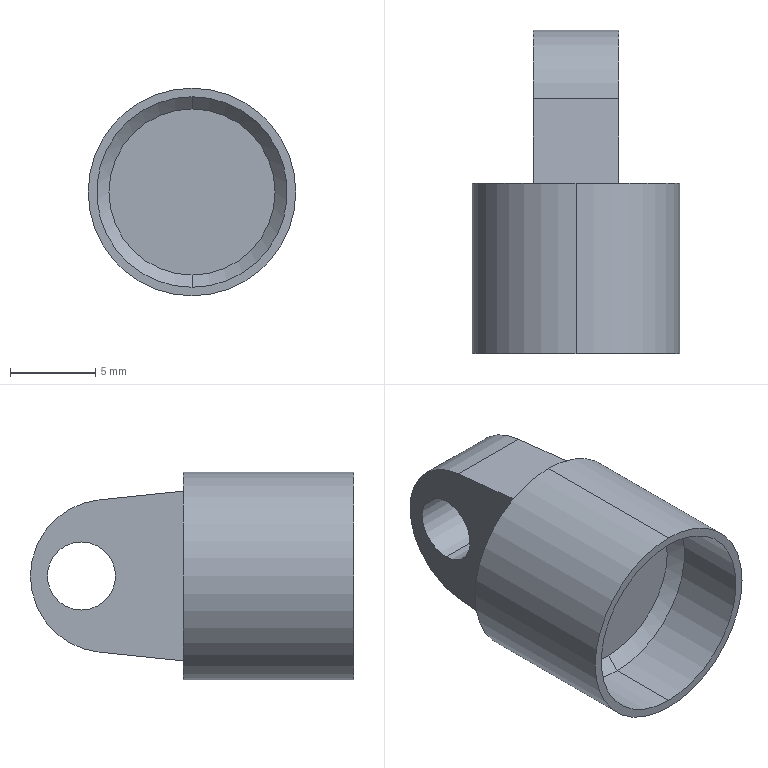Part | SolidWorks | features ICE 3, Chamfer 1, Extrusion 1 | 1 solid | 16 faces | box 12.2 x 19 x 12.2 mm | volume 995.495 mm3 | cylinder 7 | plane 7 | cone 2 | commonest cylinder face diameters 4 x2 11.2 x2 12.2 x2 9 x1
STEP:
#1=CARTESIAN_POINT('',(0.,5.,4.88));
#2=VERTEX_POINT('',#1);
#3=CARTESIAN_POINT('',(0.,5.,-4.88));
#4=VERTEX_POINT('',#3);
#5=CARTESIAN_POINT('',(0.,5.,0.));
#6=DIRECTION('',(0.,-1.,0.));
#7=DIRECTION('',(0.,0.,-1.));
#8=AXIS2_PLACEMENT_3D('',#5,#6,#7);
#9=CIRCLE('',#8,4.88);
#10=EDGE_CURVE('',#2,#4,#9,.T.);
#11=ORIENTED_EDGE('',*,*,#10,.F.);
#12=CARTESIAN_POINT('',(0.,4.28,5.6));
#13=VERTEX_POINT('',#12);
#14=CARTESIAN_POINT('',(0.,5.,4.88));
#15=DIRECTION('',(0.,-0.7071,0.7071));
#16=VECTOR('',#15,1000.);
#17=LINE('',#14,#16);
#18=EDGE_CURVE('',#2,#13,#17,.T.);
#19=ORIENTED_EDGE('',*,*,#18,.T.);
#20=CARTESIAN_POINT('',(0.,4.28,-5.6));
#21=VERTEX_POINT('',#20);
#22=CARTESIAN_POINT('',(0.,4.28,0.));
#23=DIRECTION('',(0.,1.,0.));
#24=DIRECTION('',(0.,0.,-1.));
#25=AXIS2_PLACEMENT_3D('',#22,#23,#24);
#26=CIRCLE('',#25,5.6);
#27=EDGE_CURVE('',#21,#13,#26,.T.);
#28=ORIENTED_EDGE('',*,*,#27,.F.);
#29=CARTESIAN_POINT('',(0.,5.,-4.88));
#30=DIRECTION('',(0.,-0.7071,-0.7071));
#31=VECTOR('',#30,1000.);
#32=LINE('',#29,#31);
#33=EDGE_CURVE('',#4,#21,#32,.T.);
#34=ORIENTED_EDGE('',*,*,#33,.F.);
#35=EDGE_LOOP('',(#11,#19,#28,#34));
#36=FACE_OUTER_BOUND('',#35,.T.);
#37=CARTESIAN_POINT('',(0.,5.,0.));
#38=DIRECTION('',(0.,-1.,0.));
#39=DIRECTION('',(0.,0.,-1.));
#40=AXIS2_PLACEMENT_3D('',#37,#38,#39);
#41=CONICAL_SURFACE('',#40,4.88,0.7854);
#42=ADVANCED_FACE('',(#36),#41,.F.);
#43=ORIENTED_EDGE('',*,*,#27,.T.);
#44=CARTESIAN_POINT('',(0.,0.,5.6));
#45=VERTEX_POINT('',#44);
#46=CARTESIAN_POINT('',(0.,5.,5.6));
#47=DIRECTION('',(0.,-1.,0.));
#48=VECTOR('',#47,1000.);
#49=LINE('',#46,#48);
#50=EDGE_CURVE('',#13,#45,#49,.T.);
#51=ORIENTED_EDGE('',*,*,#50,.T.);
#52=CARTESIAN_POINT('',(0.,0.,-5.6));
#53=VERTEX_POINT('',#52);
#54=CARTESIAN_POINT('',(0.,0.,0.));
#55=DIRECTION('',(0.,-1.,0.));
#56=DIRECTION('',(0.,0.,-1.));
#57=AXIS2_PLACEMENT_3D('',#54,#55,#56);
#58=CIRCLE('',#57,5.6);
#59=EDGE_CURVE('',#45,#53,#58,.T.);
#60=ORIENTED_EDGE('',*,*,#59,.T.);
#61=CARTESIAN_POINT('',(0.,5.,-5.6));
#62=DIRECTION('',(0.,-1.,0.));
#63=VECTOR('',#62,1000.);
#64=LINE('',#61,#63);
#65=EDGE_CURVE('',#21,#53,#64,.T.);
#66=ORIENTED_EDGE('',*,*,#65,.F.);
#67=EDGE_LOOP('',(#43,#51,#60,#66));
#68=FACE_OUTER_BOUND('',#67,.T.);
#69=CARTESIAN_POINT('',(0.,5.,0.));
#70=DIRECTION('',(0.,-1.,0.));
#71=DIRECTION('',(0.,0.,-1.));
#72=AXIS2_PLACEMENT_3D('',#69,#70,#71);
#73=CYLINDRICAL_SURFACE('',#72,5.6);
#74=ADVANCED_FACE('',(#68),#73,.F.);
#75=CARTESIAN_POINT('',(-2.5,16.,-2.));
#76=VERTEX_POINT('',#75);
#77=CARTESIAN_POINT('',(-2.5,16.,2.));
#78=VERTEX_POINT('',#77);
#79=CARTESIAN_POINT('',(-2.5,16.,0.));
#80=DIRECTION('',(-1.,0.,0.));
#81=DIRECTION('',(0.,0.,1.));
#82=AXIS2_PLACEMENT_3D('',#79,#80,#81);
#83=CIRCLE('',#82,2.);
#84=EDGE_CURVE('',#76,#78,#83,.T.);
#85=ORIENTED_EDGE('',*,*,#84,.T.);
#86=CARTESIAN_POINT('',(2.5,16.,2.));
#87=VERTEX_POINT('',#86);
#88=CARTESIAN_POINT('',(-6.1,16.,2.));
#89=DIRECTION('',(1.,0.,0.));
#90=VECTOR('',#89,1000.);
#91=LINE('',#88,#90);
#92=EDGE_CURVE('',#78,#87,#91,.T.);
#93=ORIENTED_EDGE('',*,*,#92,.T.);
#94=CARTESIAN_POINT('',(2.5,16.,-2.));
#95=VERTEX_POINT('',#94);
#96=CARTESIAN_POINT('',(2.5,16.,0.));
#97=DIRECTION('',(1.,0.,0.));
#98=DIRECTION('',(0.,0.,-1.));
#99=AXIS2_PLACEMENT_3D('',#96,#97,#98);
#100=CIRCLE('',#99,2.);
#101=EDGE_CURVE('',#87,#95,#100,.T.);
#102=ORIENTED_EDGE('',*,*,#101,.T.);
#103=CARTESIAN_POINT('',(-6.1,16.,-2.));
#104=DIRECTION('',(1.,0.,0.));
#105=VECTOR('',#104,1000.);
#106=LINE('',#103,#105);
#107=EDGE_CURVE('',#76,#95,#106,.T.);
#108=ORIENTED_EDGE('',*,*,#107,.F.);
#109=EDGE_LOOP('',(#85,#93,#102,#108));
#110=FACE_OUTER_BOUND('',#109,.T.);
#111=CARTESIAN_POINT('',(-6.1,16.,0.));
#112=DIRECTION('',(1.,0.,0.));
#113=DIRECTION('',(0.,0.,-1.));
#114=AXIS2_PLACEMENT_3D('',#111,#112,#113);
#115=CYLINDRICAL_SURFACE('',#114,2.);
#116=ADVANCED_FACE('',(#110),#115,.F.);
#117=CARTESIAN_POINT('',(0.,10.,6.1));
#118=VERTEX_POINT('',#117);
#119=CARTESIAN_POINT('',(0.,10.,-6.1));
#120=VERTEX_POINT('',#119);
#121=CARTESIAN_POINT('',(0.,10.,0.));
#122=DIRECTION('',(0.,1.,0.));
#123=DIRECTION('',(0.,0.,1.));
#124=AXIS2_PLACEMENT_3D('',#121,#122,#123);
#125=CIRCLE('',#124,6.1);
#126=EDGE_CURVE('',#118,#120,#125,.T.);
#127=ORIENTED_EDGE('',*,*,#126,.F.);
#128=CARTESIAN_POINT('',(0.,0.,6.1));
#129=VERTEX_POINT('',#128);
#130=CARTESIAN_POINT('',(0.,10.,6.1));
#131=DIRECTION('',(0.,-1.,0.));
#132=VECTOR('',#131,1000.);
#133=LINE('',#130,#132);
#134=EDGE_CURVE('',#118,#129,#133,.T.);
#135=ORIENTED_EDGE('',*,*,#134,.T.);
#136=CARTESIAN_POINT('',(0.,0.,-6.1));
#137=VERTEX_POINT('',#136);
#138=CARTESIAN_POINT('',(0.,0.,0.));
#139=DIRECTION('',(0.,1.,0.));
#140=DIRECTION('',(0.,0.,1.));
#141=AXIS2_PLACEMENT_3D('',#138,#139,#140);
#142=CIRCLE('',#141,6.1);
#143=EDGE_CURVE('',#129,#137,#142,.T.);
#144=ORIENTED_EDGE('',*,*,#143,.T.);
#145=CARTESIAN_POINT('',(0.,10.,-6.1));
#146=DIRECTION('',(0.,-1.,0.));
#147=VECTOR('',#146,1000.);
#148=LINE('',#145,#147);
#149=EDGE_CURVE('',#120,#137,#148,.T.);
#150=ORIENTED_EDGE('',*,*,#149,.F.);
#151=EDGE_LOOP('',(#127,#135,#144,#150));
#152=FACE_OUTER_BOUND('',#151,.T.);
#153=CARTESIAN_POINT('',(0.,10.,0.));
#154=DIRECTION('',(0.,-1.,0.));
#155=DIRECTION('',(0.,0.,-1.));
#156=AXIS2_PLACEMENT_3D('',#153,#154,#155);
#157=CYLINDRICAL_SURFACE('',#156,6.1);
#158=ADVANCED_FACE('',(#152),#157,.T.);
#159=CARTESIAN_POINT('',(0.,10.,0.));
#160=DIRECTION('',(0.,1.,0.));
#161=DIRECTION('',(0.,0.,1.));
#162=AXIS2_PLACEMENT_3D('',#159,#160,#161);
#163=CIRCLE('',#162,6.1);
#164=EDGE_CURVE('',#120,#118,#163,.T.);
#165=ORIENTED_EDGE('',*,*,#164,.T.);
#166=ORIENTED_EDGE('',*,*,#126,.T.);
#167=EDGE_LOOP('',(#165,#166));
#168=FACE_OUTER_BOUND('',#167,.T.);
#169=CARTESIAN_POINT('',(2.5,10.,4.993));
#170=VERTEX_POINT('',#169);
#171=CARTESIAN_POINT('',(-2.5,10.,4.993));
#172=VERTEX_POINT('',#171);
#173=CARTESIAN_POINT('',(2.5,10.,4.993));
#174=DIRECTION('',(-1.,0.,0.));
#175=VECTOR('',#174,1000.);
#176=LINE('',#173,#175);
#177=EDGE_CURVE('',#170,#172,#176,.T.);
#178=ORIENTED_EDGE('',*,*,#177,.T.);
#179=CARTESIAN_POINT('',(-2.5,10.,-4.993));
#180=VERTEX_POINT('',#179);
#181=CARTESIAN_POINT('',(-2.5,10.,4.993));
#182=DIRECTION('',(0.,0.,-1.));
#183=VECTOR('',#182,1000.);
#184=LINE('',#181,#183);
#185=EDGE_CURVE('',#172,#180,#184,.T.);
#186=ORIENTED_EDGE('',*,*,#185,.T.);
#187=CARTESIAN_POINT('',(2.5,10.,-4.993));
#188=VERTEX_POINT('',#187);
#189=CARTESIAN_POINT('',(2.5,10.,-4.993));
#190=DIRECTION('',(-1.,0.,0.));
#191=VECTOR('',#190,1000.);
#192=LINE('',#189,#191);
#193=EDGE_CURVE('',#188,#180,#192,.T.);
#194=ORIENTED_EDGE('',*,*,#193,.F.);
#195=CARTESIAN_POINT('',(2.5,10.,4.993));
#196=DIRECTION('',(0.,0.,-1.));
#197=VECTOR('',#196,1000.);
#198=LINE('',#195,#197);
#199=EDGE_CURVE('',#170,#188,#198,.T.);
#200=ORIENTED_EDGE('',*,*,#199,.F.);
#201=EDGE_LOOP('',(#178,#186,#194,#200));
#202=FACE_BOUND('',#201,.T.);
#203=CARTESIAN_POINT('',(0.,10.,0.));
#204=DIRECTION('',(0.,1.,0.));
#205=DIRECTION('',(0.,0.,1.));
#206=AXIS2_PLACEMENT_3D('',#203,#204,#205);
#207=PLANE('',#206);
#208=ADVANCED_FACE('',(#168,#202),#207,.T.);
#209=ORIENTED_EDGE('',*,*,#134,.F.);
#210=ORIENTED_EDGE('',*,*,#164,.F.);
#211=ORIENTED_EDGE('',*,*,#149,.T.);
#212=CARTESIAN_POINT('',(0.,0.,0.));
#213=DIRECTION('',(0.,1.,0.));
#214=DIRECTION('',(0.,0.,1.));
#215=AXIS2_PLACEMENT_3D('',#212,#213,#214);
#216=CIRCLE('',#215,6.1);
#217=EDGE_CURVE('',#137,#129,#216,.T.);
#218=ORIENTED_EDGE('',*,*,#217,.T.);
#219=EDGE_LOOP('',(#209,#210,#211,#218));
#220=FACE_OUTER_BOUND('',#219,.T.);
#221=CARTESIAN_POINT('',(0.,10.,0.));
#222=DIRECTION('',(0.,-1.,0.));
#223=DIRECTION('',(0.,0.,-1.));
#224=AXIS2_PLACEMENT_3D('',#221,#222,#223);
#225=CYLINDRICAL_SURFACE('',#224,6.1);
#226=ADVANCED_FACE('',(#220),#225,.T.);
#227=CARTESIAN_POINT('',(0.,0.,0.));
#228=DIRECTION('',(0.,-1.,0.));
#229=DIRECTION('',(0.,0.,-1.));
#230=AXIS2_PLACEMENT_3D('',#227,#228,#229);
#231=CIRCLE('',#230,5.6);
#232=EDGE_CURVE('',#53,#45,#231,.T.);
#233=ORIENTED_EDGE('',*,*,#232,.F.);
#234=ORIENTED_EDGE('',*,*,#59,.F.);
#235=EDGE_LOOP('',(#233,#234));
#236=FACE_BOUND('',#235,.T.);
#237=ORIENTED_EDGE('',*,*,#217,.F.);
#238=ORIENTED_EDGE('',*,*,#143,.F.);
#239=EDGE_LOOP('',(#237,#238));
#240=FACE_OUTER_BOUND('',#239,.T.);
#241=CARTESIAN_POINT('',(0.,0.,0.));
#242=DIRECTION('',(0.,1.,0.));
#243=DIRECTION('',(0.,0.,1.));
#244=AXIS2_PLACEMENT_3D('',#241,#242,#243);
#245=PLANE('',#244);
#246=ADVANCED_FACE('',(#236,#240),#245,.F.);
#247=CARTESIAN_POINT('',(-2.5,14.966,-4.476));
#248=VERTEX_POINT('',#247);
#249=CARTESIAN_POINT('',(-2.5,10.,-4.993));
#250=DIRECTION('',(0.,0.9946,0.1035));
#251=VECTOR('',#250,1000.);
#252=LINE('',#249,#251);
#253=EDGE_CURVE('',#180,#248,#252,.T.);
#254=ORIENTED_EDGE('',*,*,#253,.T.);
#255=CARTESIAN_POINT('',(2.5,14.966,-4.476));
#256=VERTEX_POINT('',#255);
#257=CARTESIAN_POINT('',(2.5,14.966,-4.476));
#258=DIRECTION('',(-1.,0.,0.));
#259=VECTOR('',#258,1000.);
#260=LINE('',#257,#259);
#261=EDGE_CURVE('',#256,#248,#260,.T.);
#262=ORIENTED_EDGE('',*,*,#261,.F.);
#263=CARTESIAN_POINT('',(2.5,10.,-4.993));
#264=DIRECTION('',(0.,0.9946,0.1035));
#265=VECTOR('',#264,1000.);
#266=LINE('',#263,#265);
#267=EDGE_CURVE('',#188,#256,#266,.T.);
#268=ORIENTED_EDGE('',*,*,#267,.F.);
#269=ORIENTED_EDGE('',*,*,#193,.T.);
#270=EDGE_LOOP('',(#254,#262,#268,#269));
#271=FACE_OUTER_BOUND('',#270,.T.);
#272=CARTESIAN_POINT('',(2.5,10.,-4.993));
#273=DIRECTION('',(0.,-0.1035,0.9946));
#274=DIRECTION('',(0.,-0.9946,-0.1035));
#275=AXIS2_PLACEMENT_3D('',#272,#273,#274);
#276=PLANE('',#275);
#277=ADVANCED_FACE('',(#271),#276,.F.);
#278=CARTESIAN_POINT('',(-2.5,14.966,4.476));
#279=VERTEX_POINT('',#278);
#280=CARTESIAN_POINT('',(-2.5,14.5,0.));
#281=DIRECTION('',(1.,0.,0.));
#282=DIRECTION('',(0.,0.,1.));
#283=AXIS2_PLACEMENT_3D('',#280,#281,#282);
#284=CIRCLE('',#283,4.5);
#285=EDGE_CURVE('',#248,#279,#284,.T.);
#286=ORIENTED_EDGE('',*,*,#285,.T.);
#287=CARTESIAN_POINT('',(2.5,14.966,4.476));
#288=VERTEX_POINT('',#287);
#289=CARTESIAN_POINT('',(2.5,14.966,4.476));
#290=DIRECTION('',(-1.,0.,0.));
#291=VECTOR('',#290,1000.);
#292=LINE('',#289,#291);
#293=EDGE_CURVE('',#288,#279,#292,.T.);
#294=ORIENTED_EDGE('',*,*,#293,.F.);
#295=CARTESIAN_POINT('',(2.5,14.5,0.));
#296=DIRECTION('',(1.,0.,0.));
#297=DIRECTION('',(0.,0.,1.));
#298=AXIS2_PLACEMENT_3D('',#295,#296,#297);
#299=CIRCLE('',#298,4.5);
#300=EDGE_CURVE('',#256,#288,#299,.T.);
#301=ORIENTED_EDGE('',*,*,#300,.F.);
#302=ORIENTED_EDGE('',*,*,#261,.T.);
#303=EDGE_LOOP('',(#286,#294,#301,#302));
#304=FACE_OUTER_BOUND('',#303,.T.);
#305=CARTESIAN_POINT('',(2.5,14.5,0.));
#306=DIRECTION('',(-1.,0.,0.));
#307=DIRECTION('',(0.,0.,1.));
#308=AXIS2_PLACEMENT_3D('',#305,#306,#307);
#309=CYLINDRICAL_SURFACE('',#308,4.5);
#310=ADVANCED_FACE('',(#304),#309,.T.);
#311=CARTESIAN_POINT('',(-2.5,10.,4.993));
#312=DIRECTION('',(0.,-0.9946,0.1035));
#313=VECTOR('',#312,1000.);
#314=LINE('',#311,#313);
#315=EDGE_CURVE('',#279,#172,#314,.T.);
#316=ORIENTED_EDGE('',*,*,#315,.T.);
#317=ORIENTED_EDGE('',*,*,#177,.F.);
#318=CARTESIAN_POINT('',(2.5,10.,4.993));
#319=DIRECTION('',(0.,-0.9946,0.1035));
#320=VECTOR('',#319,1000.);
#321=LINE('',#318,#320);
#322=EDGE_CURVE('',#288,#170,#321,.T.);
#323=ORIENTED_EDGE('',*,*,#322,.F.);
#324=ORIENTED_EDGE('',*,*,#293,.T.);
#325=EDGE_LOOP('',(#316,#317,#323,#324));
#326=FACE_OUTER_BOUND('',#325,.T.);
#327=CARTESIAN_POINT('',(2.5,10.,4.993));
#328=DIRECTION('',(0.,-0.1035,-0.9946));
#329=DIRECTION('',(0.,0.9946,-0.1035));
#330=AXIS2_PLACEMENT_3D('',#327,#328,#329);
#331=PLANE('',#330);
#332=ADVANCED_FACE('',(#326),#331,.F.);
#333=CARTESIAN_POINT('',(2.5,16.,0.));
#334=DIRECTION('',(1.,0.,0.));
#335=DIRECTION('',(0.,0.,-1.));
#336=AXIS2_PLACEMENT_3D('',#333,#334,#335);
#337=CIRCLE('',#336,2.);
#338=EDGE_CURVE('',#95,#87,#337,.T.);
#339=ORIENTED_EDGE('',*,*,#338,.F.);
#340=ORIENTED_EDGE('',*,*,#101,.F.);
#341=EDGE_LOOP('',(#339,#340));
#342=FACE_BOUND('',#341,.T.);
#343=ORIENTED_EDGE('',*,*,#199,.T.);
#344=ORIENTED_EDGE('',*,*,#267,.T.);
#345=ORIENTED_EDGE('',*,*,#300,.T.);
#346=ORIENTED_EDGE('',*,*,#322,.T.);
#347=EDGE_LOOP('',(#343,#344,#345,#346));
#348=FACE_OUTER_BOUND('',#347,.T.);
#349=CARTESIAN_POINT('',(2.5,14.5,0.));
#350=DIRECTION('',(-1.,0.,0.));
#351=DIRECTION('',(0.,0.,1.));
#352=AXIS2_PLACEMENT_3D('',#349,#350,#351);
#353=PLANE('',#352);
#354=ADVANCED_FACE('',(#342,#348),#353,.F.);
#355=ORIENTED_EDGE('',*,*,#84,.F.);
#356=CARTESIAN_POINT('',(-2.5,16.,0.));
#357=DIRECTION('',(-1.,0.,0.));
#358=DIRECTION('',(0.,0.,1.));
#359=AXIS2_PLACEMENT_3D('',#356,#357,#358);
#360=CIRCLE('',#359,2.);
#361=EDGE_CURVE('',#78,#76,#360,.T.);
#362=ORIENTED_EDGE('',*,*,#361,.F.);
#363=EDGE_LOOP('',(#355,#362));
#364=FACE_BOUND('',#363,.T.);
#365=ORIENTED_EDGE('',*,*,#185,.F.);
#366=ORIENTED_EDGE('',*,*,#315,.F.);
#367=ORIENTED_EDGE('',*,*,#285,.F.);
#368=ORIENTED_EDGE('',*,*,#253,.F.);
#369=EDGE_LOOP('',(#365,#366,#367,#368));
#370=FACE_OUTER_BOUND('',#369,.T.);
#371=CARTESIAN_POINT('',(-2.5,14.5,0.));
#372=DIRECTION('',(-1.,0.,0.));
#373=DIRECTION('',(0.,0.,1.));
#374=AXIS2_PLACEMENT_3D('',#371,#372,#373);
#375=PLANE('',#374);
#376=ADVANCED_FACE('',(#364,#370),#375,.T.);
#377=ORIENTED_EDGE('',*,*,#92,.F.);
#378=ORIENTED_EDGE('',*,*,#361,.T.);
#379=ORIENTED_EDGE('',*,*,#107,.T.);
#380=ORIENTED_EDGE('',*,*,#338,.T.);
#381=EDGE_LOOP('',(#377,#378,#379,#380));
#382=FACE_OUTER_BOUND('',#381,.T.);
#383=CARTESIAN_POINT('',(-6.1,16.,0.));
#384=DIRECTION('',(1.,0.,0.));
#385=DIRECTION('',(0.,0.,-1.));
#386=AXIS2_PLACEMENT_3D('',#383,#384,#385);
#387=CYLINDRICAL_SURFACE('',#386,2.);
#388=ADVANCED_FACE('',(#382),#387,.F.);
#389=ORIENTED_EDGE('',*,*,#50,.F.);
#390=CARTESIAN_POINT('',(0.,4.28,0.));
#391=DIRECTION('',(0.,1.,0.));
#392=DIRECTION('',(0.,0.,-1.));
#393=AXIS2_PLACEMENT_3D('',#390,#391,#392);
#394=CIRCLE('',#393,5.6);
#395=EDGE_CURVE('',#13,#21,#394,.T.);
#396=ORIENTED_EDGE('',*,*,#395,.T.);
#397=ORIENTED_EDGE('',*,*,#65,.T.);
#398=ORIENTED_EDGE('',*,*,#232,.T.);
#399=EDGE_LOOP('',(#389,#396,#397,#398));
#400=FACE_OUTER_BOUND('',#399,.T.);
#401=CARTESIAN_POINT('',(0.,5.,0.));
#402=DIRECTION('',(0.,-1.,0.));
#403=DIRECTION('',(0.,0.,-1.));
#404=AXIS2_PLACEMENT_3D('',#401,#402,#403);
#405=CYLINDRICAL_SURFACE('',#404,5.6);
#406=ADVANCED_FACE('',(#400),#405,.F.);
#407=CARTESIAN_POINT('',(0.,5.,0.));
#408=DIRECTION('',(0.,-1.,0.));
#409=DIRECTION('',(0.,0.,-1.));
#410=AXIS2_PLACEMENT_3D('',#407,#408,#409);
#411=CIRCLE('',#410,4.88);
#412=EDGE_CURVE('',#4,#2,#411,.T.);
#413=ORIENTED_EDGE('',*,*,#412,.T.);
#414=ORIENTED_EDGE('',*,*,#10,.T.);
#415=EDGE_LOOP('',(#413,#414));
#416=FACE_OUTER_BOUND('',#415,.T.);
#417=CARTESIAN_POINT('',(0.,5.,0.));
#418=DIRECTION('',(0.,-1.,0.));
#419=DIRECTION('',(0.,0.,-1.));
#420=AXIS2_PLACEMENT_3D('',#417,#418,#419);
#421=PLANE('',#420);
#422=ADVANCED_FACE('',(#416),#421,.T.);
#423=ORIENTED_EDGE('',*,*,#18,.F.);
#424=ORIENTED_EDGE('',*,*,#412,.F.);
#425=ORIENTED_EDGE('',*,*,#33,.T.);
#426=ORIENTED_EDGE('',*,*,#395,.F.);
#427=EDGE_LOOP('',(#423,#424,#425,#426));
#428=FACE_OUTER_BOUND('',#427,.T.);
#429=CARTESIAN_POINT('',(0.,5.,0.));
#430=DIRECTION('',(0.,-1.,0.));
#431=DIRECTION('',(0.,0.,-1.));
#432=AXIS2_PLACEMENT_3D('',#429,#430,#431);
#433=CONICAL_SURFACE('',#432,4.88,0.7854);
#434=ADVANCED_FACE('',(#428),#433,.F.);
#435=CLOSED_SHELL('',(#42,#74,#116,#158,#208,#226,#246,#277,#310,#332,#354,#376,#388,#406,#422,#434));
#436=MANIFOLD_SOLID_BREP('',#435);
#437=CARTESIAN_POINT('',(0.,0.,0.));
#438=DIRECTION('',(0.,0.,1.));
#439=DIRECTION('',(1.,0.,0.));
#440=AXIS2_PLACEMENT_3D('',#437,#438,#439);
#441=(LENGTH_UNIT()NAMED_UNIT(*)SI_UNIT(.MILLI.,.METRE.));
#442=UNCERTAINTY_MEASURE_WITH_UNIT(LENGTH_MEASURE(0.00001),#441,'','');
#443=(NAMED_UNIT(*)PLANE_ANGLE_UNIT()SI_UNIT($,.RADIAN.));
#444=(NAMED_UNIT(*)SI_UNIT($,.STERADIAN.)SOLID_ANGLE_UNIT());
#445=(GEOMETRIC_REPRESENTATION_CONTEXT(3)GLOBAL_UNCERTAINTY_ASSIGNED_CONTEXT((#442))GLOBAL_UNIT_ASSIGNED_CONTEXT((#441,#443,#444))REPRESENTATION_CONTEXT('',''));
#446=ADVANCED_BREP_SHAPE_REPRESENTATION('',(#436,#440),#445);